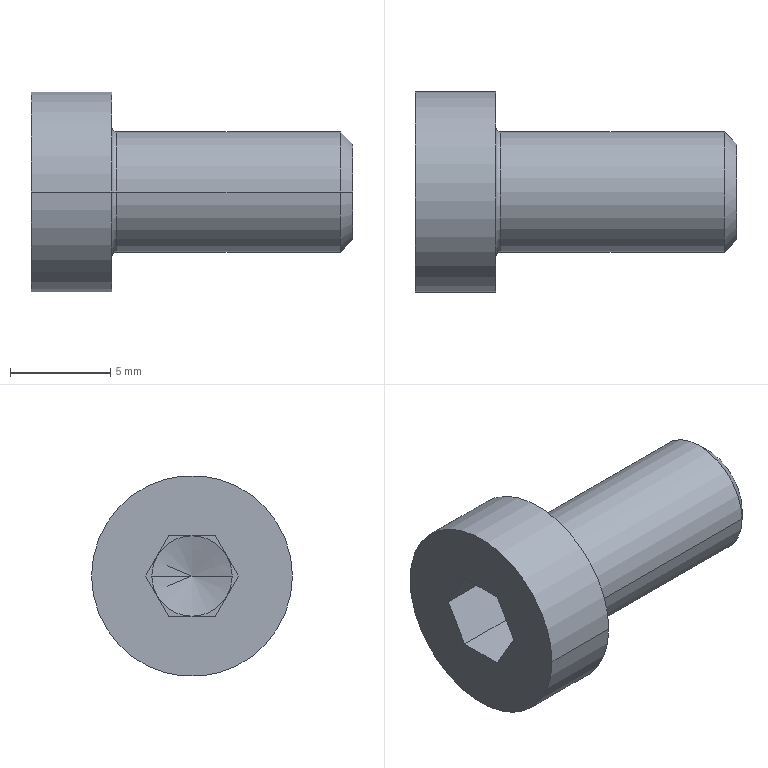Part | STEP file | CBSSTH6-12-17 | 1 solid | 25 faces | box 16 x 10 x 10 mm | volume 606.589 mm3 | plane 15 | cone 4 | cylinder 4 | torus 2 | commonest cylinder face diameters 6 x2 10 x2
STEP:
#1=CARTESIAN_POINT('',(-0.4641,0.,0.));
#2=VERTEX_POINT('',#1);
#3=CARTESIAN_POINT('',(-1.,-2.,0.));
#4=VERTEX_POINT('',#3);
#5=CARTESIAN_POINT('',(-0.4641,0.,0.));
#6=DIRECTION('',(-0.2588,-0.9659,0.));
#7=VECTOR('',#6,1000.);
#8=LINE('',#5,#7);
#9=EDGE_CURVE('',#2,#4,#8,.T.);
#10=ORIENTED_EDGE('',*,*,#9,.F.);
#11=CARTESIAN_POINT('',(-1.,2.,0.));
#12=VERTEX_POINT('',#11);
#13=CARTESIAN_POINT('',(-0.4641,0.,0.));
#14=DIRECTION('',(-0.2588,0.9659,0.));
#15=VECTOR('',#14,1000.);
#16=LINE('',#13,#15);
#17=EDGE_CURVE('',#2,#12,#16,.T.);
#18=ORIENTED_EDGE('',*,*,#17,.T.);
#19=CARTESIAN_POINT('',(-1.,1.732,-1.));
#20=VERTEX_POINT('',#19);
#21=CARTESIAN_POINT('',(-1.,0.,0.));
#22=DIRECTION('',(1.,0.,0.));
#23=DIRECTION('',(0.,1.,0.));
#24=AXIS2_PLACEMENT_3D('',#21,#22,#23);
#25=CIRCLE('',#24,2.);
#26=EDGE_CURVE('',#20,#12,#25,.T.);
#27=ORIENTED_EDGE('',*,*,#26,.F.);
#28=CARTESIAN_POINT('',(-1.,0.,-2.));
#29=VERTEX_POINT('',#28);
#30=CARTESIAN_POINT('',(-1.,0.,0.));
#31=DIRECTION('',(1.,0.,0.));
#32=DIRECTION('',(0.,1.,0.));
#33=AXIS2_PLACEMENT_3D('',#30,#31,#32);
#34=CIRCLE('',#33,2.);
#35=EDGE_CURVE('',#29,#20,#34,.T.);
#36=ORIENTED_EDGE('',*,*,#35,.F.);
#37=CARTESIAN_POINT('',(-1.,-1.732,-1.));
#38=VERTEX_POINT('',#37);
#39=CARTESIAN_POINT('',(-1.,0.,0.));
#40=DIRECTION('',(1.,0.,0.));
#41=DIRECTION('',(0.,1.,0.));
#42=AXIS2_PLACEMENT_3D('',#39,#40,#41);
#43=CIRCLE('',#42,2.);
#44=EDGE_CURVE('',#38,#29,#43,.T.);
#45=ORIENTED_EDGE('',*,*,#44,.F.);
#46=CARTESIAN_POINT('',(-1.,0.,0.));
#47=DIRECTION('',(1.,0.,0.));
#48=DIRECTION('',(0.,1.,0.));
#49=AXIS2_PLACEMENT_3D('',#46,#47,#48);
#50=CIRCLE('',#49,2.);
#51=EDGE_CURVE('',#4,#38,#50,.T.);
#52=ORIENTED_EDGE('',*,*,#51,.F.);
#53=EDGE_LOOP('',(#10,#18,#27,#36,#45,#52));
#54=FACE_OUTER_BOUND('',#53,.T.);
#55=CARTESIAN_POINT('',(-1000.464,0.,0.));
#56=DIRECTION('',(-1.,0.,0.));
#57=DIRECTION('',(0.,-1.,0.));
#58=AXIS2_PLACEMENT_3D('',#55,#56,#57);
#59=CONICAL_SURFACE('',#58,3732.051,1.309);
#60=ADVANCED_FACE('',(#54),#59,.F.);
#61=CARTESIAN_POINT('',(12.,2.387,0.));
#62=VERTEX_POINT('',#61);
#63=CARTESIAN_POINT('',(12.,-2.387,0.));
#64=VERTEX_POINT('',#63);
#65=CARTESIAN_POINT('',(12.,0.,0.));
#66=DIRECTION('',(1.,0.,0.));
#67=DIRECTION('',(0.,1.,0.));
#68=AXIS2_PLACEMENT_3D('',#65,#66,#67);
#69=CIRCLE('',#68,2.387);
#70=EDGE_CURVE('',#62,#64,#69,.T.);
#71=ORIENTED_EDGE('',*,*,#70,.F.);
#72=CARTESIAN_POINT('',(11.387,3.,0.));
#73=VERTEX_POINT('',#72);
#74=CARTESIAN_POINT('',(11.387,3.,0.));
#75=DIRECTION('',(-0.7071,0.7071,0.));
#76=VECTOR('',#75,1000.);
#77=LINE('',#74,#76);
#78=EDGE_CURVE('',#62,#73,#77,.T.);
#79=ORIENTED_EDGE('',*,*,#78,.T.);
#80=CARTESIAN_POINT('',(11.387,-3.,0.));
#81=VERTEX_POINT('',#80);
#82=CARTESIAN_POINT('',(11.387,0.,0.));
#83=DIRECTION('',(1.,0.,0.));
#84=DIRECTION('',(0.,1.,0.));
#85=AXIS2_PLACEMENT_3D('',#82,#83,#84);
#86=CIRCLE('',#85,3.);
#87=EDGE_CURVE('',#73,#81,#86,.T.);
#88=ORIENTED_EDGE('',*,*,#87,.T.);
#89=CARTESIAN_POINT('',(11.387,-3.,0.));
#90=DIRECTION('',(-0.7071,-0.7071,0.));
#91=VECTOR('',#90,1000.);
#92=LINE('',#89,#91);
#93=EDGE_CURVE('',#64,#81,#92,.T.);
#94=ORIENTED_EDGE('',*,*,#93,.F.);
#95=EDGE_LOOP('',(#71,#79,#88,#94));
#96=FACE_OUTER_BOUND('',#95,.T.);
#97=CARTESIAN_POINT('',(11.387,0.,0.));
#98=DIRECTION('',(-1.,0.,0.));
#99=DIRECTION('',(0.,-1.,0.));
#100=AXIS2_PLACEMENT_3D('',#97,#98,#99);
#101=CONICAL_SURFACE('',#100,3.,0.7854);
#102=ADVANCED_FACE('',(#96),#101,.T.);
#103=CARTESIAN_POINT('',(0.25,3.,0.));
#104=VERTEX_POINT('',#103);
#105=CARTESIAN_POINT('',(0.25,-3.,0.));
#106=VERTEX_POINT('',#105);
#107=CARTESIAN_POINT('',(0.25,0.,0.));
#108=DIRECTION('',(1.,0.,0.));
#109=DIRECTION('',(0.,1.,0.));
#110=AXIS2_PLACEMENT_3D('',#107,#108,#109);
#111=CIRCLE('',#110,3.);
#112=EDGE_CURVE('',#104,#106,#111,.T.);
#113=ORIENTED_EDGE('',*,*,#112,.T.);
#114=CARTESIAN_POINT('',(16.,-3.,0.));
#115=DIRECTION('',(1.,0.,0.));
#116=VECTOR('',#115,1000.);
#117=LINE('',#114,#116);
#118=EDGE_CURVE('',#106,#81,#117,.T.);
#119=ORIENTED_EDGE('',*,*,#118,.T.);
#120=ORIENTED_EDGE('',*,*,#87,.F.);
#121=CARTESIAN_POINT('',(16.,3.,0.));
#122=DIRECTION('',(1.,0.,0.));
#123=VECTOR('',#122,1000.);
#124=LINE('',#121,#123);
#125=EDGE_CURVE('',#104,#73,#124,.T.);
#126=ORIENTED_EDGE('',*,*,#125,.F.);
#127=EDGE_LOOP('',(#113,#119,#120,#126));
#128=FACE_OUTER_BOUND('',#127,.T.);
#129=CARTESIAN_POINT('',(16.,0.,0.));
#130=DIRECTION('',(1.,0.,0.));
#131=DIRECTION('',(0.,1.,0.));
#132=AXIS2_PLACEMENT_3D('',#129,#130,#131);
#133=CYLINDRICAL_SURFACE('',#132,3.);
#134=ADVANCED_FACE('',(#128),#133,.T.);
#135=CARTESIAN_POINT('',(0.25,0.,0.));
#136=DIRECTION('',(1.,0.,0.));
#137=DIRECTION('',(0.,1.,0.));
#138=AXIS2_PLACEMENT_3D('',#135,#136,#137);
#139=CIRCLE('',#138,3.);
#140=EDGE_CURVE('',#106,#104,#139,.T.);
#141=ORIENTED_EDGE('',*,*,#140,.F.);
#142=CARTESIAN_POINT('',(0.,-3.25,0.));
#143=VERTEX_POINT('',#142);
#144=CARTESIAN_POINT('',(0.25,-3.25,0.));
#145=DIRECTION('',(0.,0.,1.));
#146=DIRECTION('',(0.,-1.,0.));
#147=AXIS2_PLACEMENT_3D('',#144,#145,#146);
#148=CIRCLE('',#147,0.25);
#149=EDGE_CURVE('',#106,#143,#148,.T.);
#150=ORIENTED_EDGE('',*,*,#149,.T.);
#151=CARTESIAN_POINT('',(0.,3.25,0.));
#152=VERTEX_POINT('',#151);
#153=CARTESIAN_POINT('',(0.,0.,0.));
#154=DIRECTION('',(1.,0.,0.));
#155=DIRECTION('',(0.,1.,0.));
#156=AXIS2_PLACEMENT_3D('',#153,#154,#155);
#157=CIRCLE('',#156,3.25);
#158=EDGE_CURVE('',#143,#152,#157,.T.);
#159=ORIENTED_EDGE('',*,*,#158,.T.);
#160=CARTESIAN_POINT('',(0.25,3.25,0.));
#161=DIRECTION('',(0.,0.,-1.));
#162=DIRECTION('',(-1.,0.,0.));
#163=AXIS2_PLACEMENT_3D('',#160,#161,#162);
#164=CIRCLE('',#163,0.25);
#165=EDGE_CURVE('',#104,#152,#164,.T.);
#166=ORIENTED_EDGE('',*,*,#165,.F.);
#167=EDGE_LOOP('',(#141,#150,#159,#166));
#168=FACE_OUTER_BOUND('',#167,.T.);
#169=CARTESIAN_POINT('',(0.25,0.,0.));
#170=DIRECTION('',(1.,0.,0.));
#171=DIRECTION('',(0.,1.,0.));
#172=AXIS2_PLACEMENT_3D('',#169,#170,#171);
#173=TOROIDAL_SURFACE('',#172,3.25,0.25);
#174=ADVANCED_FACE('',(#168),#173,.F.);
#175=CARTESIAN_POINT('',(-4.,5.,0.));
#176=VERTEX_POINT('',#175);
#177=CARTESIAN_POINT('',(-4.,-5.,0.));
#178=VERTEX_POINT('',#177);
#179=CARTESIAN_POINT('',(-4.,0.,0.));
#180=DIRECTION('',(1.,0.,0.));
#181=DIRECTION('',(0.,1.,0.));
#182=AXIS2_PLACEMENT_3D('',#179,#180,#181);
#183=CIRCLE('',#182,5.);
#184=EDGE_CURVE('',#176,#178,#183,.T.);
#185=ORIENTED_EDGE('',*,*,#184,.T.);
#186=CARTESIAN_POINT('',(0.,-5.,0.));
#187=VERTEX_POINT('',#186);
#188=CARTESIAN_POINT('',(16.,-5.,0.));
#189=DIRECTION('',(1.,0.,0.));
#190=VECTOR('',#189,1000.);
#191=LINE('',#188,#190);
#192=EDGE_CURVE('',#178,#187,#191,.T.);
#193=ORIENTED_EDGE('',*,*,#192,.T.);
#194=CARTESIAN_POINT('',(0.,5.,0.));
#195=VERTEX_POINT('',#194);
#196=CARTESIAN_POINT('',(0.,0.,0.));
#197=DIRECTION('',(1.,0.,0.));
#198=DIRECTION('',(0.,1.,0.));
#199=AXIS2_PLACEMENT_3D('',#196,#197,#198);
#200=CIRCLE('',#199,5.);
#201=EDGE_CURVE('',#195,#187,#200,.T.);
#202=ORIENTED_EDGE('',*,*,#201,.F.);
#203=CARTESIAN_POINT('',(16.,5.,0.));
#204=DIRECTION('',(1.,0.,0.));
#205=VECTOR('',#204,1000.);
#206=LINE('',#203,#205);
#207=EDGE_CURVE('',#176,#195,#206,.T.);
#208=ORIENTED_EDGE('',*,*,#207,.F.);
#209=EDGE_LOOP('',(#185,#193,#202,#208));
#210=FACE_OUTER_BOUND('',#209,.T.);
#211=CARTESIAN_POINT('',(16.,0.,0.));
#212=DIRECTION('',(1.,0.,0.));
#213=DIRECTION('',(0.,1.,0.));
#214=AXIS2_PLACEMENT_3D('',#211,#212,#213);
#215=CYLINDRICAL_SURFACE('',#214,5.);
#216=ADVANCED_FACE('',(#210),#215,.T.);
#217=ORIENTED_EDGE('',*,*,#184,.F.);
#218=CARTESIAN_POINT('',(-4.,0.,0.));
#219=DIRECTION('',(1.,0.,0.));
#220=DIRECTION('',(0.,1.,0.));
#221=AXIS2_PLACEMENT_3D('',#218,#219,#220);
#222=CIRCLE('',#221,5.);
#223=EDGE_CURVE('',#178,#176,#222,.T.);
#224=ORIENTED_EDGE('',*,*,#223,.F.);
#225=EDGE_LOOP('',(#217,#224));
#226=FACE_OUTER_BOUND('',#225,.T.);
#227=CARTESIAN_POINT('',(-4.,-1.155,-2.));
#228=VERTEX_POINT('',#227);
#229=CARTESIAN_POINT('',(-4.,-2.309,0.));
#230=VERTEX_POINT('',#229);
#231=CARTESIAN_POINT('',(-4.,-1.232,-1.866));
#232=DIRECTION('',(0.,-0.5,0.866));
#233=VECTOR('',#232,1000.);
#234=LINE('',#231,#233);
#235=EDGE_CURVE('',#228,#230,#234,.T.);
#236=ORIENTED_EDGE('',*,*,#235,.F.);
#237=CARTESIAN_POINT('',(-4.,1.155,-2.));
#238=VERTEX_POINT('',#237);
#239=CARTESIAN_POINT('',(-4.,2.,-2.));
#240=DIRECTION('',(0.,-1.,0.));
#241=VECTOR('',#240,1000.);
#242=LINE('',#239,#241);
#243=EDGE_CURVE('',#238,#228,#242,.T.);
#244=ORIENTED_EDGE('',*,*,#243,.F.);
#245=CARTESIAN_POINT('',(-4.,2.309,0.));
#246=VERTEX_POINT('',#245);
#247=CARTESIAN_POINT('',(-4.,2.232,-0.134));
#248=DIRECTION('',(0.,-0.5,-0.866));
#249=VECTOR('',#248,1000.);
#250=LINE('',#247,#249);
#251=EDGE_CURVE('',#246,#238,#250,.T.);
#252=ORIENTED_EDGE('',*,*,#251,.F.);
#253=CARTESIAN_POINT('',(-4.,1.155,2.));
#254=VERTEX_POINT('',#253);
#255=CARTESIAN_POINT('',(-4.,2.232,0.134));
#256=DIRECTION('',(0.,0.5,-0.866));
#257=VECTOR('',#256,1000.);
#258=LINE('',#255,#257);
#259=EDGE_CURVE('',#254,#246,#258,.T.);
#260=ORIENTED_EDGE('',*,*,#259,.F.);
#261=CARTESIAN_POINT('',(-4.,-1.155,2.));
#262=VERTEX_POINT('',#261);
#263=CARTESIAN_POINT('',(-4.,2.,2.));
#264=DIRECTION('',(0.,1.,0.));
#265=VECTOR('',#264,1000.);
#266=LINE('',#263,#265);
#267=EDGE_CURVE('',#262,#254,#266,.T.);
#268=ORIENTED_EDGE('',*,*,#267,.F.);
#269=CARTESIAN_POINT('',(-4.,-1.232,1.866));
#270=DIRECTION('',(0.,0.5,0.866));
#271=VECTOR('',#270,1000.);
#272=LINE('',#269,#271);
#273=EDGE_CURVE('',#230,#262,#272,.T.);
#274=ORIENTED_EDGE('',*,*,#273,.F.);
#275=EDGE_LOOP('',(#236,#244,#252,#260,#268,#274));
#276=FACE_BOUND('',#275,.T.);
#277=CARTESIAN_POINT('',(-4.,2.,0.));
#278=DIRECTION('',(1.,0.,0.));
#279=DIRECTION('',(0.,1.,0.));
#280=AXIS2_PLACEMENT_3D('',#277,#278,#279);
#281=PLANE('',#280);
#282=ADVANCED_FACE('',(#226,#276),#281,.F.);
#283=ORIENTED_EDGE('',*,*,#192,.F.);
#284=ORIENTED_EDGE('',*,*,#223,.T.);
#285=ORIENTED_EDGE('',*,*,#207,.T.);
#286=CARTESIAN_POINT('',(0.,0.,0.));
#287=DIRECTION('',(1.,0.,0.));
#288=DIRECTION('',(0.,1.,0.));
#289=AXIS2_PLACEMENT_3D('',#286,#287,#288);
#290=CIRCLE('',#289,5.);
#291=EDGE_CURVE('',#187,#195,#290,.T.);
#292=ORIENTED_EDGE('',*,*,#291,.F.);
#293=EDGE_LOOP('',(#283,#284,#285,#292));
#294=FACE_OUTER_BOUND('',#293,.T.);
#295=CARTESIAN_POINT('',(16.,0.,0.));
#296=DIRECTION('',(1.,0.,0.));
#297=DIRECTION('',(0.,1.,0.));
#298=AXIS2_PLACEMENT_3D('',#295,#296,#297);
#299=CYLINDRICAL_SURFACE('',#298,5.);
#300=ADVANCED_FACE('',(#294),#299,.T.);
#301=CARTESIAN_POINT('',(0.,0.,0.));
#302=DIRECTION('',(1.,0.,0.));
#303=DIRECTION('',(0.,1.,0.));
#304=AXIS2_PLACEMENT_3D('',#301,#302,#303);
#305=CIRCLE('',#304,3.25);
#306=EDGE_CURVE('',#152,#143,#305,.T.);
#307=ORIENTED_EDGE('',*,*,#306,.F.);
#308=ORIENTED_EDGE('',*,*,#158,.F.);
#309=EDGE_LOOP('',(#307,#308));
#310=FACE_BOUND('',#309,.T.);
#311=ORIENTED_EDGE('',*,*,#201,.T.);
#312=ORIENTED_EDGE('',*,*,#291,.T.);
#313=EDGE_LOOP('',(#311,#312));
#314=FACE_OUTER_BOUND('',#313,.T.);
#315=CARTESIAN_POINT('',(0.,5.,0.));
#316=DIRECTION('',(-1.,0.,0.));
#317=DIRECTION('',(0.,-1.,0.));
#318=AXIS2_PLACEMENT_3D('',#315,#316,#317);
#319=PLANE('',#318);
#320=ADVANCED_FACE('',(#310,#314),#319,.F.);
#321=ORIENTED_EDGE('',*,*,#149,.F.);
#322=ORIENTED_EDGE('',*,*,#112,.F.);
#323=ORIENTED_EDGE('',*,*,#165,.T.);
#324=ORIENTED_EDGE('',*,*,#306,.T.);
#325=EDGE_LOOP('',(#321,#322,#323,#324));
#326=FACE_OUTER_BOUND('',#325,.T.);
#327=CARTESIAN_POINT('',(0.25,0.,0.));
#328=DIRECTION('',(1.,0.,0.));
#329=DIRECTION('',(0.,1.,0.));
#330=AXIS2_PLACEMENT_3D('',#327,#328,#329);
#331=TOROIDAL_SURFACE('',#330,3.25,0.25);
#332=ADVANCED_FACE('',(#326),#331,.F.);
#333=ORIENTED_EDGE('',*,*,#118,.F.);
#334=ORIENTED_EDGE('',*,*,#140,.T.);
#335=ORIENTED_EDGE('',*,*,#125,.T.);
#336=CARTESIAN_POINT('',(11.387,0.,0.));
#337=DIRECTION('',(1.,0.,0.));
#338=DIRECTION('',(0.,1.,0.));
#339=AXIS2_PLACEMENT_3D('',#336,#337,#338);
#340=CIRCLE('',#339,3.);
#341=EDGE_CURVE('',#81,#73,#340,.T.);
#342=ORIENTED_EDGE('',*,*,#341,.F.);
#343=EDGE_LOOP('',(#333,#334,#335,#342));
#344=FACE_OUTER_BOUND('',#343,.T.);
#345=CARTESIAN_POINT('',(16.,0.,0.));
#346=DIRECTION('',(1.,0.,0.));
#347=DIRECTION('',(0.,1.,0.));
#348=AXIS2_PLACEMENT_3D('',#345,#346,#347);
#349=CYLINDRICAL_SURFACE('',#348,3.);
#350=ADVANCED_FACE('',(#344),#349,.T.);
#351=ORIENTED_EDGE('',*,*,#78,.F.);
#352=CARTESIAN_POINT('',(12.,0.,0.));
#353=DIRECTION('',(1.,0.,0.));
#354=DIRECTION('',(0.,1.,0.));
#355=AXIS2_PLACEMENT_3D('',#352,#353,#354);
#356=CIRCLE('',#355,2.387);
#357=EDGE_CURVE('',#64,#62,#356,.T.);
#358=ORIENTED_EDGE('',*,*,#357,.F.);
#359=ORIENTED_EDGE('',*,*,#93,.T.);
#360=ORIENTED_EDGE('',*,*,#341,.T.);
#361=EDGE_LOOP('',(#351,#358,#359,#360));
#362=FACE_OUTER_BOUND('',#361,.T.);
#363=CARTESIAN_POINT('',(11.387,0.,0.));
#364=DIRECTION('',(-1.,0.,0.));
#365=DIRECTION('',(0.,-1.,0.));
#366=AXIS2_PLACEMENT_3D('',#363,#364,#365);
#367=CONICAL_SURFACE('',#366,3.,0.7854);
#368=ADVANCED_FACE('',(#362),#367,.T.);
#369=ORIENTED_EDGE('',*,*,#357,.T.);
#370=ORIENTED_EDGE('',*,*,#70,.T.);
#371=EDGE_LOOP('',(#369,#370));
#372=FACE_OUTER_BOUND('',#371,.T.);
#373=CARTESIAN_POINT('',(12.,2.387,0.));
#374=DIRECTION('',(-1.,0.,0.));
#375=DIRECTION('',(0.,-1.,0.));
#376=AXIS2_PLACEMENT_3D('',#373,#374,#375);
#377=PLANE('',#376);
#378=ADVANCED_FACE('',(#372),#377,.F.);
#379=CARTESIAN_POINT('',(-1.,-1.155,-2.));
#380=VERTEX_POINT('',#379);
#381=CARTESIAN_POINT('',(-1.,-1.155,-2.));
#382=DIRECTION('',(0.,1.,0.));
#383=VECTOR('',#382,1000.);
#384=LINE('',#381,#383);
#385=EDGE_CURVE('',#380,#29,#384,.T.);
#386=ORIENTED_EDGE('',*,*,#385,.F.);
#387=CARTESIAN_POINT('',(-1.,-2.309,0.));
#388=DIRECTION('',(0.,0.5,-0.866));
#389=VECTOR('',#388,1000.);
#390=LINE('',#387,#389);
#391=EDGE_CURVE('',#38,#380,#390,.T.);
#392=ORIENTED_EDGE('',*,*,#391,.F.);
#393=ORIENTED_EDGE('',*,*,#44,.T.);
#394=EDGE_LOOP('',(#386,#392,#393));
#395=FACE_OUTER_BOUND('',#394,.T.);
#396=CARTESIAN_POINT('',(-1.,0.,0.));
#397=DIRECTION('',(1.,0.,0.));
#398=DIRECTION('',(0.,0.,-1.));
#399=AXIS2_PLACEMENT_3D('',#396,#397,#398);
#400=PLANE('',#399);
#401=ADVANCED_FACE('',(#395),#400,.F.);
#402=CARTESIAN_POINT('',(-1.,-2.309,0.));
#403=VERTEX_POINT('',#402);
#404=CARTESIAN_POINT('',(-1.,-2.309,0.));
#405=DIRECTION('',(0.,0.5,-0.866));
#406=VECTOR('',#405,1000.);
#407=LINE('',#404,#406);
#408=EDGE_CURVE('',#403,#38,#407,.T.);
#409=ORIENTED_EDGE('',*,*,#408,.F.);
#410=CARTESIAN_POINT('',(-1.,-1.732,1.));
#411=VERTEX_POINT('',#410);
#412=CARTESIAN_POINT('',(-1.,-1.155,2.));
#413=DIRECTION('',(0.,-0.5,-0.866));
#414=VECTOR('',#413,1000.);
#415=LINE('',#412,#414);
#416=EDGE_CURVE('',#411,#403,#415,.T.);
#417=ORIENTED_EDGE('',*,*,#416,.F.);
#418=CARTESIAN_POINT('',(-1.,0.,0.));
#419=DIRECTION('',(1.,0.,0.));
#420=DIRECTION('',(0.,1.,0.));
#421=AXIS2_PLACEMENT_3D('',#418,#419,#420);
#422=CIRCLE('',#421,2.);
#423=EDGE_CURVE('',#411,#4,#422,.T.);
#424=ORIENTED_EDGE('',*,*,#423,.T.);
#425=ORIENTED_EDGE('',*,*,#51,.T.);
#426=EDGE_LOOP('',(#409,#417,#424,#425));
#427=FACE_OUTER_BOUND('',#426,.T.);
#428=CARTESIAN_POINT('',(-1.,0.,0.));
#429=DIRECTION('',(1.,0.,0.));
#430=DIRECTION('',(0.,0.,-1.));
#431=AXIS2_PLACEMENT_3D('',#428,#429,#430);
#432=PLANE('',#431);
#433=ADVANCED_FACE('',(#427),#432,.F.);
#434=CARTESIAN_POINT('',(-1.,-1.155,2.));
#435=VERTEX_POINT('',#434);
#436=CARTESIAN_POINT('',(-1.,-1.155,2.));
#437=DIRECTION('',(0.,-0.5,-0.866));
#438=VECTOR('',#437,1000.);
#439=LINE('',#436,#438);
#440=EDGE_CURVE('',#435,#411,#439,.T.);
#441=ORIENTED_EDGE('',*,*,#440,.F.);
#442=CARTESIAN_POINT('',(-1.,0.,2.));
#443=VERTEX_POINT('',#442);
#444=CARTESIAN_POINT('',(-1.,1.155,2.));
#445=DIRECTION('',(0.,-1.,0.));
#446=VECTOR('',#445,1000.);
#447=LINE('',#444,#446);
#448=EDGE_CURVE('',#443,#435,#447,.T.);
#449=ORIENTED_EDGE('',*,*,#448,.F.);
#450=CARTESIAN_POINT('',(-1.,0.,0.));
#451=DIRECTION('',(1.,0.,0.));
#452=DIRECTION('',(0.,1.,0.));
#453=AXIS2_PLACEMENT_3D('',#450,#451,#452);
#454=CIRCLE('',#453,2.);
#455=EDGE_CURVE('',#443,#411,#454,.T.);
#456=ORIENTED_EDGE('',*,*,#455,.T.);
#457=EDGE_LOOP('',(#441,#449,#456));
#458=FACE_OUTER_BOUND('',#457,.T.);
#459=CARTESIAN_POINT('',(-1.,0.,0.));
#460=DIRECTION('',(1.,0.,0.));
#461=DIRECTION('',(0.,0.,-1.));
#462=AXIS2_PLACEMENT_3D('',#459,#460,#461);
#463=PLANE('',#462);
#464=ADVANCED_FACE('',(#458),#463,.F.);
#465=CARTESIAN_POINT('',(-1.,1.155,2.));
#466=VERTEX_POINT('',#465);
#467=CARTESIAN_POINT('',(-1.,1.155,2.));
#468=DIRECTION('',(0.,-1.,0.));
#469=VECTOR('',#468,1000.);
#470=LINE('',#467,#469);
#471=EDGE_CURVE('',#466,#443,#470,.T.);
#472=ORIENTED_EDGE('',*,*,#471,.F.);
#473=CARTESIAN_POINT('',(-1.,1.732,1.));
#474=VERTEX_POINT('',#473);
#475=CARTESIAN_POINT('',(-1.,2.309,0.));
#476=DIRECTION('',(0.,-0.5,0.866));
#477=VECTOR('',#476,1000.);
#478=LINE('',#475,#477);
#479=EDGE_CURVE('',#474,#466,#478,.T.);
#480=ORIENTED_EDGE('',*,*,#479,.F.);
#481=CARTESIAN_POINT('',(-1.,0.,0.));
#482=DIRECTION('',(1.,0.,0.));
#483=DIRECTION('',(0.,1.,0.));
#484=AXIS2_PLACEMENT_3D('',#481,#482,#483);
#485=CIRCLE('',#484,2.);
#486=EDGE_CURVE('',#474,#443,#485,.T.);
#487=ORIENTED_EDGE('',*,*,#486,.T.);
#488=EDGE_LOOP('',(#472,#480,#487));
#489=FACE_OUTER_BOUND('',#488,.T.);
#490=CARTESIAN_POINT('',(-1.,0.,0.));
#491=DIRECTION('',(1.,0.,0.));
#492=DIRECTION('',(0.,0.,-1.));
#493=AXIS2_PLACEMENT_3D('',#490,#491,#492);
#494=PLANE('',#493);
#495=ADVANCED_FACE('',(#489),#494,.F.);
#496=CARTESIAN_POINT('',(-1.,2.309,0.));
#497=VERTEX_POINT('',#496);
#498=CARTESIAN_POINT('',(-1.,2.309,0.));
#499=DIRECTION('',(0.,-0.5,0.866));
#500=VECTOR('',#499,1000.);
#501=LINE('',#498,#500);
#502=EDGE_CURVE('',#497,#474,#501,.T.);
#503=ORIENTED_EDGE('',*,*,#502,.F.);
#504=CARTESIAN_POINT('',(-1.,1.155,-2.));
#505=DIRECTION('',(0.,0.5,0.866));
#506=VECTOR('',#505,1000.);
#507=LINE('',#504,#506);
#508=EDGE_CURVE('',#20,#497,#507,.T.);
#509=ORIENTED_EDGE('',*,*,#508,.F.);
#510=ORIENTED_EDGE('',*,*,#26,.T.);
#511=CARTESIAN_POINT('',(-1.,0.,0.));
#512=DIRECTION('',(1.,0.,0.));
#513=DIRECTION('',(0.,1.,0.));
#514=AXIS2_PLACEMENT_3D('',#511,#512,#513);
#515=CIRCLE('',#514,2.);
#516=EDGE_CURVE('',#12,#474,#515,.T.);
#517=ORIENTED_EDGE('',*,*,#516,.T.);
#518=EDGE_LOOP('',(#503,#509,#510,#517));
#519=FACE_OUTER_BOUND('',#518,.T.);
#520=CARTESIAN_POINT('',(-1.,0.,0.));
#521=DIRECTION('',(1.,0.,0.));
#522=DIRECTION('',(0.,0.,-1.));
#523=AXIS2_PLACEMENT_3D('',#520,#521,#522);
#524=PLANE('',#523);
#525=ADVANCED_FACE('',(#519),#524,.F.);
#526=CARTESIAN_POINT('',(-1.,1.155,-2.));
#527=VERTEX_POINT('',#526);
#528=CARTESIAN_POINT('',(-1.,1.155,-2.));
#529=DIRECTION('',(0.,0.5,0.866));
#530=VECTOR('',#529,1000.);
#531=LINE('',#528,#530);
#532=EDGE_CURVE('',#527,#20,#531,.T.);
#533=ORIENTED_EDGE('',*,*,#532,.F.);
#534=CARTESIAN_POINT('',(-1.,-1.155,-2.));
#535=DIRECTION('',(0.,1.,0.));
#536=VECTOR('',#535,1000.);
#537=LINE('',#534,#536);
#538=EDGE_CURVE('',#29,#527,#537,.T.);
#539=ORIENTED_EDGE('',*,*,#538,.F.);
#540=ORIENTED_EDGE('',*,*,#35,.T.);
#541=EDGE_LOOP('',(#533,#539,#540));
#542=FACE_OUTER_BOUND('',#541,.T.);
#543=CARTESIAN_POINT('',(-1.,0.,0.));
#544=DIRECTION('',(1.,0.,0.));
#545=DIRECTION('',(0.,0.,-1.));
#546=AXIS2_PLACEMENT_3D('',#543,#544,#545);
#547=PLANE('',#546);
#548=ADVANCED_FACE('',(#542),#547,.F.);
#549=ORIENTED_EDGE('',*,*,#471,.T.);
#550=ORIENTED_EDGE('',*,*,#448,.T.);
#551=CARTESIAN_POINT('',(-1.,-1.155,2.));
#552=DIRECTION('',(-1.,0.,0.));
#553=VECTOR('',#552,1000.);
#554=LINE('',#551,#553);
#555=EDGE_CURVE('',#435,#262,#554,.T.);
#556=ORIENTED_EDGE('',*,*,#555,.T.);
#557=ORIENTED_EDGE('',*,*,#267,.T.);
#558=CARTESIAN_POINT('',(-1.,1.155,2.));
#559=DIRECTION('',(-1.,0.,0.));
#560=VECTOR('',#559,1000.);
#561=LINE('',#558,#560);
#562=EDGE_CURVE('',#466,#254,#561,.T.);
#563=ORIENTED_EDGE('',*,*,#562,.F.);
#564=EDGE_LOOP('',(#549,#550,#556,#557,#563));
#565=FACE_OUTER_BOUND('',#564,.T.);
#566=CARTESIAN_POINT('',(-1.,1.155,2.));
#567=DIRECTION('',(0.,0.,-1.));
#568=DIRECTION('',(-1.,0.,0.));
#569=AXIS2_PLACEMENT_3D('',#566,#567,#568);
#570=PLANE('',#569);
#571=ADVANCED_FACE('',(#565),#570,.T.);
#572=ORIENTED_EDGE('',*,*,#440,.T.);
#573=ORIENTED_EDGE('',*,*,#416,.T.);
#574=CARTESIAN_POINT('',(-1.,-2.309,0.));
#575=DIRECTION('',(-1.,0.,0.));
#576=VECTOR('',#575,1000.);
#577=LINE('',#574,#576);
#578=EDGE_CURVE('',#403,#230,#577,.T.);
#579=ORIENTED_EDGE('',*,*,#578,.T.);
#580=ORIENTED_EDGE('',*,*,#273,.T.);
#581=ORIENTED_EDGE('',*,*,#555,.F.);
#582=EDGE_LOOP('',(#572,#573,#579,#580,#581));
#583=FACE_OUTER_BOUND('',#582,.T.);
#584=CARTESIAN_POINT('',(-1.,-1.155,2.));
#585=DIRECTION('',(0.,0.866,-0.5));
#586=DIRECTION('',(0.,0.5,0.866));
#587=AXIS2_PLACEMENT_3D('',#584,#585,#586);
#588=PLANE('',#587);
#589=ADVANCED_FACE('',(#583),#588,.T.);
#590=ORIENTED_EDGE('',*,*,#408,.T.);
#591=ORIENTED_EDGE('',*,*,#391,.T.);
#592=CARTESIAN_POINT('',(-1.,-1.155,-2.));
#593=DIRECTION('',(-1.,0.,0.));
#594=VECTOR('',#593,1000.);
#595=LINE('',#592,#594);
#596=EDGE_CURVE('',#380,#228,#595,.T.);
#597=ORIENTED_EDGE('',*,*,#596,.T.);
#598=ORIENTED_EDGE('',*,*,#235,.T.);
#599=ORIENTED_EDGE('',*,*,#578,.F.);
#600=EDGE_LOOP('',(#590,#591,#597,#598,#599));
#601=FACE_OUTER_BOUND('',#600,.T.);
#602=CARTESIAN_POINT('',(-1.,-2.309,0.));
#603=DIRECTION('',(0.,0.866,0.5));
#604=DIRECTION('',(0.,-0.5,0.866));
#605=AXIS2_PLACEMENT_3D('',#602,#603,#604);
#606=PLANE('',#605);
#607=ADVANCED_FACE('',(#601),#606,.T.);
#608=ORIENTED_EDGE('',*,*,#385,.T.);
#609=ORIENTED_EDGE('',*,*,#538,.T.);
#610=CARTESIAN_POINT('',(-1.,1.155,-2.));
#611=DIRECTION('',(-1.,0.,0.));
#612=VECTOR('',#611,1000.);
#613=LINE('',#610,#612);
#614=EDGE_CURVE('',#527,#238,#613,.T.);
#615=ORIENTED_EDGE('',*,*,#614,.T.);
#616=ORIENTED_EDGE('',*,*,#243,.T.);
#617=ORIENTED_EDGE('',*,*,#596,.F.);
#618=EDGE_LOOP('',(#608,#609,#615,#616,#617));
#619=FACE_OUTER_BOUND('',#618,.T.);
#620=CARTESIAN_POINT('',(-1.,-1.155,-2.));
#621=DIRECTION('',(0.,0.,1.));
#622=DIRECTION('',(1.,0.,0.));
#623=AXIS2_PLACEMENT_3D('',#620,#621,#622);
#624=PLANE('',#623);
#625=ADVANCED_FACE('',(#619),#624,.T.);
#626=ORIENTED_EDGE('',*,*,#532,.T.);
#627=ORIENTED_EDGE('',*,*,#508,.T.);
#628=CARTESIAN_POINT('',(-1.,2.309,0.));
#629=DIRECTION('',(-1.,0.,0.));
#630=VECTOR('',#629,1000.);
#631=LINE('',#628,#630);
#632=EDGE_CURVE('',#497,#246,#631,.T.);
#633=ORIENTED_EDGE('',*,*,#632,.T.);
#634=ORIENTED_EDGE('',*,*,#251,.T.);
#635=ORIENTED_EDGE('',*,*,#614,.F.);
#636=EDGE_LOOP('',(#626,#627,#633,#634,#635));
#637=FACE_OUTER_BOUND('',#636,.T.);
#638=CARTESIAN_POINT('',(-1.,1.155,-2.));
#639=DIRECTION('',(0.,-0.866,0.5));
#640=DIRECTION('',(0.,-0.5,-0.866));
#641=AXIS2_PLACEMENT_3D('',#638,#639,#640);
#642=PLANE('',#641);
#643=ADVANCED_FACE('',(#637),#642,.T.);
#644=ORIENTED_EDGE('',*,*,#502,.T.);
#645=ORIENTED_EDGE('',*,*,#479,.T.);
#646=ORIENTED_EDGE('',*,*,#562,.T.);
#647=ORIENTED_EDGE('',*,*,#259,.T.);
#648=ORIENTED_EDGE('',*,*,#632,.F.);
#649=EDGE_LOOP('',(#644,#645,#646,#647,#648));
#650=FACE_OUTER_BOUND('',#649,.T.);
#651=CARTESIAN_POINT('',(-1.,2.309,0.));
#652=DIRECTION('',(0.,-0.866,-0.5));
#653=DIRECTION('',(0.,0.5,-0.866));
#654=AXIS2_PLACEMENT_3D('',#651,#652,#653);
#655=PLANE('',#654);
#656=ADVANCED_FACE('',(#650),#655,.T.);
#657=ORIENTED_EDGE('',*,*,#17,.F.);
#658=ORIENTED_EDGE('',*,*,#9,.T.);
#659=ORIENTED_EDGE('',*,*,#423,.F.);
#660=ORIENTED_EDGE('',*,*,#455,.F.);
#661=ORIENTED_EDGE('',*,*,#486,.F.);
#662=ORIENTED_EDGE('',*,*,#516,.F.);
#663=EDGE_LOOP('',(#657,#658,#659,#660,#661,#662));
#664=FACE_OUTER_BOUND('',#663,.T.);
#665=CARTESIAN_POINT('',(-1000.464,0.,0.));
#666=DIRECTION('',(-1.,0.,0.));
#667=DIRECTION('',(0.,-1.,0.));
#668=AXIS2_PLACEMENT_3D('',#665,#666,#667);
#669=CONICAL_SURFACE('',#668,3732.051,1.309);
#670=ADVANCED_FACE('',(#664),#669,.F.);
#671=CLOSED_SHELL('',(#60,#102,#134,#174,#216,#282,#300,#320,#332,#350,#368,#378,#401,#433,#464,#495,#525,#548,#571,#589,#607,#625,#643,#656,#670));
#672=MANIFOLD_SOLID_BREP('',#671);
#673=CARTESIAN_POINT('',(0.,0.,0.));
#674=DIRECTION('',(0.,0.,1.));
#675=DIRECTION('',(1.,0.,0.));
#676=AXIS2_PLACEMENT_3D('',#673,#674,#675);
#677=(LENGTH_UNIT()NAMED_UNIT(*)SI_UNIT(.MILLI.,.METRE.));
#678=UNCERTAINTY_MEASURE_WITH_UNIT(LENGTH_MEASURE(0.00001),#677,'','');
#679=(NAMED_UNIT(*)PLANE_ANGLE_UNIT()SI_UNIT($,.RADIAN.));
#680=(NAMED_UNIT(*)SI_UNIT($,.STERADIAN.)SOLID_ANGLE_UNIT());
#681=(GEOMETRIC_REPRESENTATION_CONTEXT(3)GLOBAL_UNCERTAINTY_ASSIGNED_CONTEXT((#678))GLOBAL_UNIT_ASSIGNED_CONTEXT((#677,#679,#680))REPRESENTATION_CONTEXT('',''));
#682=ADVANCED_BREP_SHAPE_REPRESENTATION('',(#672,#676),#681);